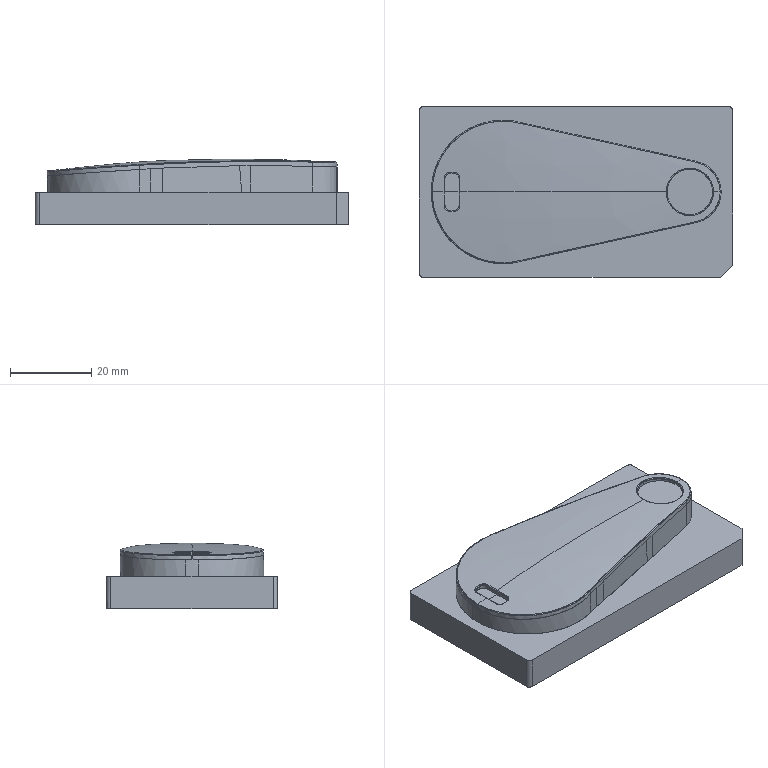NC program | PowerMill | posted with a generic post | part box 77 x 42 x 16.114 mm
Lines 5294 to 6286 of 134652:
N5391 M6
N5392 S18000 M03
N5393 G00 G90 X0.0 Y0.0
N5394 G43 Z9.8037 H2
N5395
N5396 G05 P10000 R4
N5397 X15.985 Y-10.5899
N5398 Z0.6702
N5399 G01 Z-0.5298 F3600.0
N5400 X15.9918 Y-10.569 F6000.0
N5401 G03 X15.8642 Y-10.3197 I-0.1884 J0.0609
N5402 G01 X14.5797 Y-9.9049
N5403 X12.3216 Y-10.2491
N5404 X11.9573 Y-10.2786
N5405 X10.9812 Y-10.2096
N5406 X10.4931 Y-10.2127
N5407 X7.0768 Y-10.0469
N5408 X4.1484 Y-9.3347
N5409 X3.9914 Y-9.273
N5410 X3.6604 Y-9.2133
N5411 X2.1962 Y-8.8365
N5412 X1.7082 Y-8.6326
N5413 X1.0155 Y-8.2969
N5414 X-0.244 Y-7.5021
N5415 X-2.5439 Y-5.8566
N5416 X-3.1723 Y-5.1878
N5417 X-3.8658 Y-3.9044
N5418 X-4.3321 Y-2.9283
N5419 X-4.5131 Y-2.4403
N5420 X-4.7814 Y-0.9761
N5421 X-4.9965 Y-0.4881
N5422 X-5.0691 Y0.0
N5423 X-4.9959 Y0.4881
N5424 X-4.8279 Y0.9761
N5425 X-4.5833 Y2.4403
N5426 X-4.4398 Y2.9283
N5427 X-4.1608 Y3.4164
N5428 X-3.9472 Y3.9044
N5429 X-3.6589 Y4.3925
N5430 X-2.9454 Y5.3686
N5431 X-2.4721 Y5.8566
N5432 X-1.8096 Y6.3447
N5433 X-1.7082 Y6.4511
N5434 X-0.7321 Y7.2006
N5435 X-0.6069 Y7.3208
N5436 X-0.244 Y7.5702
N5437 X0.0485 Y7.8088
N5438 X0.7321 Y8.2556
N5439 X1.2201 Y8.4464
N5440 X2.6843 Y8.9279
N5441 X3.8434 Y9.273
N5442 X4.1484 Y9.3944
N5443 X5.1246 Y9.6928
N5444 X9.517 Y10.2816
N5445 X10.0051 Y10.274
N5446 X13.9095 Y10.115
N5447 X14.3976 Y10.0238
N5448 X15.5346 Y9.7611
N5449 X15.8617 Y9.7088
N5450 X18.302 Y9.1742
N5451 X18.79 Y9.0002
N5452 X20.2542 Y8.3815
N5453 X21.2303 Y7.8837
N5454 X22.6945 Y6.9767
N5455 X23.1825 Y6.6438
N5456 X23.4753 Y6.3447
N5457 X23.6706 Y6.2105
N5458 X24.0366 Y5.8566
N5459 X24.1586 Y5.7858
N5460 X24.9777 Y4.8805
N5461 X25.1347 Y4.6324
N5462 X25.242 Y4.3925
N5463 X25.3717 Y3.9044
N5464 X25.353 Y3.4164
N5465 X25.2134 Y2.9283
N5466 X24.9263 Y2.4403
N5467 X24.4521 Y1.4642
N5468 X24.3007 Y0.9761
N5469 X24.2171 Y0.4881
N5470 X24.1864 Y0.0
N5471 X24.2177 Y-0.4881
N5472 X24.3007 Y-0.9761
N5473 X24.4552 Y-1.4642
N5474 X24.9263 Y-2.4403
N5475 X24.9304 Y-2.4473
N5476 X24.9305 Y-2.4474
N5477 X25.2136 Y-2.9283
N5478 X25.353 Y-3.4164
N5479 X25.3717 Y-3.9044
N5480 X25.242 Y-4.3925
N5481 X24.9792 Y-4.8805
N5482 X24.0229 Y-5.8566
N5483 X23.1825 Y-6.5896
N5484 X22.8614 Y-6.8327
N5485 X22.6945 Y-6.9955
N5486 X22.2064 Y-7.3451
N5487 X21.2303 Y-7.8982
N5488 X20.4067 Y-8.2969
N5489 X17.3259 Y-9.4493
N5490 X16.8378 Y-9.5607
N5491 X14.5797 Y-9.9049
N5492 X16.8369 Y-13.1705 Z-0.7226
N5493 X16.8424 Y-13.1492
N5494 G03 X16.7 Y-12.9081 I-0.1918 J0.0494
N5495 G01 X15.1386 Y-12.5061
N5496 X12.0144 Y-13.1774
N5497 X10.0051 Y-13.5276
N5498 X9.517 Y-13.568
N5499 X8.5409 Y-13.533
N5500 X7.0768 Y-13.4407
N5501 X4.6365 Y-13.0863
N5502 X2.1962 Y-12.7016
N5503 X0.7321 Y-12.2384
N5504 X-2.1962 Y-11.2009
N5505 X-2.6843 Y-10.9564
N5506 X-3.9445 Y-10.2491
N5507 X-4.6365 Y-9.7451
N5508 X-6.4624 Y-8.2969
N5509 X-7.0768 Y-7.7594
N5510 X-7.5648 Y-7.1197
N5511 X-8.6785 Y-5.3686
N5512 X-8.9342 Y-4.8805
N5513 X-9.2841 Y-3.9044
N5514 X-9.7154 Y-2.4403
N5515 X-9.9892 Y0.0
N5516 X-9.9391 Y0.4881
N5517 X-9.8428 Y0.9761
N5518 X-9.4645 Y3.4164
N5519 X-9.3065 Y3.9044
N5520 X-8.5409 Y5.4879
N5521 X-8.0529 Y6.3656
N5522 X-7.7369 Y6.8409
N5523 X-7.4278 Y7.3208
N5524 X-7.0568 Y7.8088
N5525 X-5.6126 Y9.013
N5526 X-4.0115 Y10.2491
N5527 X-3.6604 Y10.4585
N5528 X-2.6843 Y10.9644
N5529 X-0.8483 Y11.7133
N5530 X-0.7321 Y11.7403
N5531 X0.7321 Y12.3023
N5532 X1.7082 Y12.5616
N5533 X4.9711 Y13.1774
N5534 X6.1007 Y13.3217
N5535 X7.0768 Y13.4029
N5536 X8.0529 Y13.5085
N5537 X9.517 Y13.5892
N5538 X10.0051 Y13.5348
N5539 X11.9573 Y13.1885
N5540 X19.2781 Y11.6167
N5541 X24.1586 Y10.4886
N5542 X26.1108 Y9.9407
N5543 X26.4488 Y9.7611
N5544 X27.1222 Y9.273
N5545 X27.575 Y8.8486
N5546 X28.063 Y8.443
N5547 X28.683 Y7.8088
N5548 X29.4948 Y6.8327
N5549 X29.7043 Y6.3447
N5550 X29.814 Y5.8566
N5551 X29.7755 Y5.3686
N5552 X29.5272 Y4.8397
N5553 X29.1792 Y4.3925
N5554 X29.0391 Y4.301
N5555 X28.5511 Y4.0585
N5556 X27.0869 Y3.7026
N5557 X26.5989 Y3.5189
N5558 X26.1108 Y3.2616
N5559 X25.6228 Y2.9149
N5560 X25.1468 Y2.4403
N5561 X24.7984 Y1.9522
N5562 X24.5421 Y1.4642
N5563 X24.3764 Y0.9761
N5564 X24.2788 Y0.4881
N5565 X24.2425 Y0.0
N5566 X24.2788 Y-0.4881
N5567 X24.3765 Y-0.9761
N5568 X24.5432 Y-1.4642
N5569 X24.7985 Y-1.9522
N5570 X25.1347 Y-2.4286
N5571 X25.6228 Y-2.9134
N5572 X26.1108 Y-3.2612
N5573 X26.5989 Y-3.5183
N5574 X27.0869 Y-3.7067
N5575 X28.5511 Y-4.0483
N5576 X29.1791 Y-4.3925
N5577 X29.5803 Y-4.8805
N5578 X29.7754 Y-5.3686
N5579 X29.814 Y-5.8566
N5580 X29.7043 Y-6.3447
N5581 X29.5272 Y-6.7695
N5582 X29.0391 Y-7.3983
N5583 X28.6841 Y-7.8088
N5584 X28.1703 Y-8.2969
N5585 X28.063 Y-8.4416
N5586 X27.6707 Y-8.7849
N5587 X27.6697 Y-8.7859
N5588 X27.6687 Y-8.7868
N5589 X27.0869 Y-9.3106
N5590 X26.5989 Y-9.663
N5591 X26.1108 Y-9.9234
N5592 X25.6228 Y-10.0928
N5593 X24.1586 Y-10.4881
N5594 X19.2781 Y-11.6167
N5595 X15.1386 Y-12.5061
N5596 G00 Z3.4146
N5597 G01 X17.275 Y13.0315 F10000.0
N5598 G00 Z0.2846
N5599 G01 Z-0.9154 F3600.0
N5600 X17.2276 Y12.8167 F6000.0
N5601 X17.0818 Y12.1556
N5602 X24.6467 Y10.4877
N5603 X29.9536 Y9.273
N5604 X30.9913 Y8.9558
N5605 X31.9675 Y8.5409
N5606 X32.4555 Y8.2603
N5607 X32.9436 Y7.918
N5608 X33.4316 Y7.5167
N5609 X33.5949 Y7.3208
N5610 X33.8585 Y6.8327
N5611 X34.4758 Y5.3686
N5612 X34.9257 Y3.9044
N5613 X35.1649 Y2.9283
N5614 X35.2875 Y1.9522
N5615 X35.1493 Y1.4642
N5616 X34.9156 Y0.9761
N5617 X34.8958 Y0.8721
N5618 X34.4708 Y0.4881
N5619 X33.9197 Y0.215
N5620 X33.4316 Y0.1634
N5621 X32.9436 Y0.2235
N5622 X32.4555 Y0.3991
N5623 X32.4506 Y0.4188
N5624 X32.4467 Y0.4294
N5625 X32.4201 Y0.486
N5626 X32.3764 Y0.5308
N5627 X31.9675 Y0.8373
N5628 X31.4794 Y1.7222
N5629 X30.9913 Y2.3765
N5630 X30.5033 Y2.8523
N5631 X30.0152 Y3.1826
N5632 X29.5424 Y3.4164
N5633 X29.0391 Y3.6018
N5634 X28.5511 Y3.6981
N5635 X28.063 Y3.7356
N5636 X27.575 Y3.7096
N5637 X27.0869 Y3.6248
N5638 X26.5989 Y3.4707
N5639 X26.1108 Y3.2307
N5640 X25.6228 Y2.8981
N5641 X25.1347 Y2.4185
N5642 X24.7984 Y1.9522
N5643 X24.5424 Y1.4642
N5644 X24.3764 Y0.9761
N5645 X24.2788 Y0.4881
N5646 X24.2426 Y0.0
N5647 X24.2788 Y-0.4881
N5648 X24.3772 Y-0.9761
N5649 X24.5432 Y-1.4642
N5650 X24.7985 Y-1.9522
N5651 X25.1347 Y-2.4184
N5652 X25.6228 Y-2.8979
N5653 X26.1108 Y-3.2305
N5654 X26.475 Y-3.4164
N5655 X27.0869 Y-3.6228
N5656 X27.575 Y-3.7119
N5657 X28.063 Y-3.7355
N5658 X28.5511 Y-3.698
N5659 X29.0391 Y-3.6021
N5660 X29.5272 Y-3.4234
N5661 X29.7739 Y-3.3015
N5662 X28.8728 Y-1.5202
N5663 G02 X26.4134 Y-0.079 I-0.7654 J1.513
N5664 G02 X29.4882 Y0.9768 I1.694 J0.0718
N5665 G01 X29.8264 Y0.5023
N5666 G02 X29.8634 Y-0.3695 I-0.6515 J-0.4643
N5667 G01 X29.5665 Y-0.8709
N5668 G02 X28.8728 Y-1.5202 I-1.4591 J0.8636
N5669 G01 X29.7739 Y-3.3015
N5670 X30.0152 Y-3.1823
N5671 X30.4068 Y-2.9283
N5672 X30.9913 Y-2.3765
N5673 X31.4794 Y-1.7204
N5674 X31.9675 Y-0.8398
N5675 X32.3709 Y-0.5353
N5676 X32.4316 Y-0.4594
N5677 X32.4555 Y-0.3651
N5678 X32.9436 Y-0.2045
N5679 X33.4316 Y-0.1634
N5680 X33.9197 Y-0.191
N5681 X34.4077 Y-0.4074
N5682 X34.4708 Y-0.4881
N5683 X34.8958 Y-0.849
N5684 X34.9156 Y-0.9761
N5685 X35.1493 Y-1.4642
N5686 X35.2875 Y-1.9522
N5687 X35.1649 Y-2.9283
N5688 X35.0597 Y-3.4164
N5689 X34.7979 Y-4.3925
N5690 X34.4598 Y-5.3686
N5691 X34.0347 Y-6.3447
N5692 X33.8585 Y-6.8327
N5693 X33.5928 Y-7.3208
N5694 X33.4316 Y-7.5089
N5695 X33.0925 Y-7.8088
N5696 X32.4555 Y-8.2608
N5697 X31.9675 Y-8.5383
N5698 X30.9913 Y-8.9558
N5699 X30.0152 Y-9.2567
N5700 X25.1347 Y-10.3776
N5701 X16.8378 Y-12.2122
N5702 X5.6833 Y-14.6416
N5703 X3.1992 Y-15.1296
N5704 X1.7082 Y-15.3289
N5705 X0.7321 Y-15.1863
N5706 X-1.7082 Y-14.5815
N5707 X-2.6843 Y-14.2589
N5708 X-3.1723 Y-14.0252
N5709 X-6.1007 Y-12.7616
N5710 X-6.2158 Y-12.6894
N5711 X-6.5887 Y-12.5321
N5712 X-7.0768 Y-12.2223
N5713 X-7.667 Y-11.7133
N5714 X-8.827 Y-10.7372
N5715 X-9.8957 Y-9.7611
N5716 X-10.9812 Y-8.4414
N5717 X-11.0562 Y-8.2969
N5718 X-11.7166 Y-7.3208
N5719 X-11.9306 Y-6.8327
N5720 X-12.7269 Y-4.8805
N5721 X-13.2966 Y-2.4403
N5722 X-13.5318 Y0.0
N5723 X-13.1339 Y3.4164
N5724 X-13.0265 Y3.9044
N5725 X-12.8615 Y4.3925
N5726 X-12.2761 Y5.8566
N5727 X-12.055 Y6.3447
N5728 X-11.7014 Y7.3208
N5729 X-10.9812 Y8.4367
N5730 X-9.8961 Y9.7611
N5731 X-8.5409 Y11.038
N5732 X-7.5648 Y11.828
N5733 X-6.5887 Y12.5307
N5734 X-5.8996 Y12.8597
N5735 X-5.2052 Y13.1774
N5736 X-4.6365 Y13.4642
N5737 X-3.1723 Y14.0914
N5738 X-2.6843 Y14.2619
N5739 X-1.2201 Y14.7024
N5740 X0.7321 Y15.1868
N5741 X1.7082 Y15.3272
N5742 X3.1993 Y15.1296
N5743 X5.6126 Y14.6558
N5744 X9.517 Y13.8236
N5745 X17.0818 Y12.1556
N5746 X17.2276 Y12.8167
N5747 X15.8751 Y13.4159 Z-1.1082
N5748 X15.8612 Y13.3988
N5749 G03 X15.8905 Y13.1203 I0.1539 J-0.1246
N5750 G01 X17.0818 Y12.1556
N5751 X24.6467 Y10.4876
N5752 X24.6863 Y10.4785
N5753 X30.0152 Y9.3046
N5754 X30.9913 Y9.0315
N5755 X31.6504 Y8.7849
N5756 X32.6485 Y8.2969
N5757 X33.4316 Y7.7973
N5758 X33.9197 Y7.4266
N5759 X34.4077 Y7.0097
N5760 X34.8958 Y6.5253
N5761 X35.3838 Y5.9587
N5762 X35.8719 Y5.2894
N5763 X36.3599 Y4.4639
N5764 X36.6313 Y3.9044
N5765 X36.8292 Y3.4164
N5766 X37.14 Y2.4403
N5767 X37.336 Y1.4964
N5768 X37.4396 Y0.4881
N5769 Y-0.4881
N5770 X37.3407 Y-1.4642
N5771 X37.14 Y-2.4403
N5772 X36.848 Y-3.3763
N5773 X36.6333 Y-3.9044
N5774 X36.3599 Y-4.4656
N5775 X35.8719 Y-5.2895
N5776 X35.4636 Y-5.8566
N5777 X35.0579 Y-6.3447
N5778 X34.5953 Y-6.8327
N5779 X33.9197 Y-7.4274
N5780 X33.4142 Y-7.8088
N5781 X32.6481 Y-8.2969
N5782 X31.6504 Y-8.7849
N5783 X30.9913 Y-9.0294
N5784 X30.1471 Y-9.273
N5785 X22.667 Y-10.9232
N5786 X16.8378 Y-12.2122
N5787 X15.7729 Y-12.4441
N5788 X2.1962 Y-15.4393
N5789 X-1.0126 Y-16.1057
N5790 X-2.6843 Y-16.4045
N5791 X-3.6604 Y-16.4871
N5792 X-4.1484 Y-16.4057
N5793 X-6.1007 Y-15.7378
N5794 X-6.5887 Y-15.5486
N5795 X-8.0529 Y-14.7887
N5796 X-9.029 Y-14.2443
N5797 X-9.1208 Y-14.1535
N5798 X-10.4931 Y-13.2448
N5799 X-10.9812 Y-12.8331
N5800 X-11.9573 Y-11.8789
N5801 X-13.4214 Y-10.0394
N5802 X-13.9095 Y-9.3592
N5803 X-14.5184 Y-8.2969
N5804 X-14.8856 Y-7.4935
N5805 X-15.1491 Y-6.8327
N5806 X-15.2816 Y-6.3447
N5807 X-15.3737 Y-6.1218
N5808 X-15.5986 Y-5.3686
N5809 X-15.8576 Y-4.3925
N5810 X-16.21 Y-2.4403
N5811 X-16.3345 Y-0.4881
N5812 X-16.3888 Y0.0
N5813 X-16.1063 Y3.4164
N5814 X-16.004 Y3.9044
N5815 X-15.3737 Y6.0853
N5816 X-15.2688 Y6.3447
N5817 X-15.162 Y6.8327
N5818 X-14.9821 Y7.3208
N5819 X-14.5212 Y8.2969
N5820 X-14.3976 Y8.4951
N5821 X-14.267 Y8.7849
N5822 X-13.656 Y9.7611
N5823 X-12.9317 Y10.7372
N5824 X-12.4453 Y11.3284
N5825 X-11.4692 Y12.4066
N5826 X-10.5858 Y13.1774
N5827 X-9.517 Y13.9309
N5828 X-9.1208 Y14.1535
N5829 X-9.029 Y14.2299
N5830 X-8.5409 Y14.5124
N5831 X-6.5887 Y15.5482
N5832 X-6.1007 Y15.7373
N5833 X-4.1484 Y16.4125
N5834 X-3.6604 Y16.488
N5835 X-2.6843 Y16.4081
N5836 X-1.0125 Y16.1057
N5837 X1.2201 Y15.6479
N5838 X9.0502 Y13.923
N5839 X9.0508 Y13.9229
N5840 X9.517 Y13.8235
N5841 X17.0818 Y12.1556
N5842 X15.8812 Y13.4173 Z-1.301
N5843 X15.8674 Y13.4002
N5844 G03 X15.8967 Y13.1218 I0.1539 J-0.1245
N5845 G01 X17.0831 Y12.1613
N5846 X30.0152 Y9.3118
N5847 X30.5033 Y9.1853
N5848 X30.8379 Y9.0744
N5849 X30.8423 Y9.0732
N5850 X31.2509 Y8.9418
N5851 X31.6504 Y8.7849
N5852 X31.7504 Y8.736
N5853 X32.4555 Y8.4084
N5854 X32.9436 Y8.1319
N5855 X33.4337 Y7.8088
N5856 X34.0717 Y7.3208
N5857 X34.3732 Y7.0391
N5858 X34.4077 Y7.0097
N5859 X34.4548 Y6.963
N5860 X34.8958 Y6.551
N5861 X35.3838 Y5.9928
N5862 X35.8719 Y5.3332
N5863 X36.3599 Y4.5207
N5864 X36.6659 Y3.9044
N5865 X36.848 Y3.4634
N5866 X37.1824 Y2.4403
N5867 X37.3851 Y1.4642
N5868 X37.487 Y0.4881
N5869 X37.4872 Y-0.4881
N5870 X37.3871 Y-1.4642
N5871 X37.1852 Y-2.4403
N5872 X37.0358 Y-2.9283
N5873 X36.6659 Y-3.9044
N5874 X36.3599 Y-4.5218
N5875 X35.8457 Y-5.3686
N5876 X35.4887 Y-5.8566
N5877 X34.8958 Y-6.551
N5878 X34.6122 Y-6.8327
N5879 X34.0705 Y-7.3208
N5880 X33.4316 Y-7.8121
N5881 X32.9436 Y-8.1319
N5882 X32.4555 Y-8.4084
N5883 X31.6685 Y-8.7849
N5884 X30.9913 Y-9.0374
N5885 X30.0152 Y-9.3119
N5886 X-3.0263 Y-16.5938
N5887 X-5.3877 Y-17.0818
N5888 X-7.0768 Y-17.3569
N5889 X-7.5648 Y-17.3933
N5890 X-8.0529 Y-17.3741
N5891 X-8.5409 Y-17.2194
N5892 X-9.8825 Y-16.5938
N5893 X-10.4931 Y-16.2662
N5894 X-11.5234 Y-15.6177
N5895 X-12.8694 Y-14.6416
N5896 X-13.4893 Y-14.1535
N5897 X-14.388 Y-13.1774
N5898 X-15.5219 Y-11.7133
N5899 X-16.3498 Y-10.2735
N5900 X-16.6683 Y-9.7611
N5901 X-16.9285 Y-9.273
N5902 X-17.8139 Y-7.1013
N5903 X-17.8962 Y-6.8327
N5904 X-17.9805 Y-6.3447
N5905 X-18.2202 Y-5.3686
N5906 X-18.4325 Y-4.3925
N5907 X-18.7084 Y-2.4403
N5908 X-18.8098 Y-0.4881
N5909 X-18.8636 Y0.0
N5910 X-18.6188 Y3.4164
N5911 X-18.5192 Y3.9044
N5912 X-17.9635 Y6.3447
N5913 X-17.8966 Y6.8327
N5914 X-17.8139 Y7.1013
N5915 X-17.3259 Y8.3813
N5916 X-16.9288 Y9.273
N5917 X-16.1465 Y10.7372
N5918 X-15.5346 Y11.7133
N5919 X-15.196 Y12.2013
N5920 X-14.8856 Y12.5959
N5921 X-13.9095 Y13.7109
N5922 X-12.4453 Y14.9669
N5923 X-11.5309 Y15.6177
N5924 X-10.4931 Y16.289
N5925 X-8.5409 Y17.224
N5926 X-8.0529 Y17.3748
N5927 X-7.5648 Y17.3896
N5928 X-7.0768 Y17.3569
N5929 X-5.6126 Y17.1212
N5930 X-3.1723 Y16.6245
N5931 X17.0831 Y12.1613
N5932 X15.87 Y13.4318 Z-1.4939
N5933 X15.8561 Y13.4147
N5934 G03 X15.8855 Y13.1363 I0.154 J-0.1245
N5935 G01 X17.0842 Y12.1662
N5936 X30.0152 Y9.3187
N5937 X30.5033 Y9.1912
N5938 X30.9652 Y9.0388
N5939 X30.9913 Y9.0314
N5940 X31.0211 Y9.0203
N5941 X31.4794 Y8.8691
N5942 X32.4555 Y8.4161
N5943 X32.9436 Y8.1397
N5944 X33.4417 Y7.8088
N5945 X33.9197 Y7.4538
N5946 X34.4077 Y7.0364
N5947 X34.8958 Y6.5609
N5948 X35.3838 Y6.0032
N5949 X35.8554 Y5.3686
N5950 X36.3599 Y4.5357
N5951 X36.6741 Y3.9044
N5952 X36.8711 Y3.4164
N5953 X37.1923 Y2.4403
N5954 X37.336 Y1.79
N5955 X37.3789 Y1.4936
N5956 X37.385 Y1.4642
N5957 X37.3898 Y1.4181
N5958 X37.4538 Y0.9761
N5959 X37.4754 Y0.5983
N5960 X37.4866 Y0.4952
N5961 X37.4873 Y0.3916
N5962 X37.5097 Y0.0
N5963 X37.4927 Y-0.4881
N5964 X37.3944 Y-1.4642
N5965 X37.1922 Y-2.4403
N5966 X37.045 Y-2.9283
N5967 X36.6741 Y-3.9044
N5968 X36.3599 Y-4.536
N5969 X35.8719 Y-5.3449
N5970 X35.4966 Y-5.8566
N5971 X34.8958 Y-6.5608
N5972 X34.4077 Y-7.0366
N5973 X34.0809 Y-7.3208
N5974 X33.4464 Y-7.8088
N5975 X32.9436 Y-8.1397
N5976 X32.4555 Y-8.4161
N5977 X31.6849 Y-8.7849
N5978 X30.9913 Y-9.0449
N5979 X30.0152 Y-9.3187
N5980 X-7.4559 Y-17.5699
N5981 X-9.029 Y-17.8917
N5982 X-9.76 Y-18.0169
N5983 X-10.4931 Y-18.1296
N5984 X-10.9812 Y-18.1485
N5985 X-11.4692 Y-18.1366
N5986 X-11.7996 Y-18.0579
N5987 X-11.9573 Y-17.9896
N5988 X-12.9334 Y-17.4587
N5989 X-14.8113 Y-16.1057
N5990 X-15.4001 Y-15.6177
N5991 X-16.3591 Y-14.6416
N5992 X-17.1793 Y-13.6655
N5993 X-17.5114 Y-13.1774
N5994 X-18.3798 Y-11.7133
N5995 X-18.6318 Y-11.2252
N5996 X-18.8262 Y-10.7372
N5997 X-19.4761 Y-9.273
N5998 X-20.2686 Y-6.8327
N5999 X-20.7217 Y-4.3925
N6000 X-20.9442 Y-2.4403
N6001 X-21.0669 Y0.0
N6002 X-20.8559 Y3.4164
N6003 X-20.2594 Y6.8327
N6004 X-19.9799 Y7.8088
N6005 X-19.6459 Y8.7849
N6006 X-19.0892 Y10.2491
N6007 X-18.393 Y11.7133
N6008 X-17.8139 Y12.7014
N6009 X-17.3259 Y13.448
N6010 X-16.3341 Y14.6416
N6011 X-15.878 Y15.1296
N6012 X-14.8856 Y16.0714
N6013 X-13.9095 Y16.8229
N6014 X-12.4453 Y17.7241
N6015 X-11.9573 Y17.9898
N6016 X-11.4692 Y18.1338
N6017 X-10.9812 Y18.1508
N6018 X-10.4931 Y18.1286
N6019 X-9.029 Y17.8905
N6020 X-7.4559 Y17.5699
N6021 X17.0842 Y12.1662
N6022 X15.8638 Y13.4435 Z-1.6867
N6023 X15.85 Y13.4264
N6024 G03 X15.8794 Y13.1479 I0.1539 J-0.1246
N6025 G01 X17.0854 Y12.1719
N6026 X30.0152 Y9.3256
N6027 X30.5033 Y9.1981
N6028 X31.4794 Y8.8762
N6029 X32.4555 Y8.4238
N6030 X32.9436 Y8.1475
N6031 X33.1484 Y8.0036
N6032 X33.1505 Y8.0022
N6033 X33.5386 Y7.7369
N6034 X33.9197 Y7.4616
N6035 X34.4077 Y7.0459
N6036 X34.8958 Y6.5707
N6037 X35.3838 Y6.0136
N6038 X35.8636 Y5.3686
N6039 X36.3599 Y4.5507
N6040 X36.6817 Y3.9044
N6041 X36.8786 Y3.4164
N6042 X37.1993 Y2.4403
N6043 X37.336 Y1.822
N6044 X37.4594 Y0.9761
N6045 X37.5165 Y0.0
N6046 X37.4967 Y-0.3735
N6047 X37.4927 Y-0.488
N6048 X37.4883 Y-0.5317
N6049 X37.4647 Y-0.9761
N6050 X37.4014 Y-1.4642
N6051 X37.1992 Y-2.4403
N6052 X37.0519 Y-2.9283
N6053 X36.6817 Y-3.9044
N6054 X36.3599 Y-4.5512
N6055 X35.8719 Y-5.3566
N6056 X35.505 Y-5.8566
N6057 X34.8958 Y-6.5707
N6058 X34.4963 Y-6.9486
N6059 X34.0913 Y-7.3208
N6060 X33.4316 Y-7.8245
N6061 X32.9436 Y-8.1475
N6062 X32.4555 Y-8.4238
N6063 X31.7014 Y-8.7849
N6064 X30.9913 Y-9.052
N6065 X30.0152 Y-9.3256
N6066 X-10.0051 Y-18.1367
N6067 X-11.9652 Y-18.546
N6068 X-13.4214 Y-18.8225
N6069 X-13.9095 Y-18.8456
N6070 X-14.3976 Y-18.8271
N6071 X-14.8856 Y-18.6811
N6072 X-15.1294 Y-18.546
N6073 X-15.8617 Y-18.0621
N6074 X-16.8378 Y-17.3034
N6075 X-18.5155 Y-15.6177
N6076 X-18.9206 Y-15.1296
N6077 X-19.8962 Y-13.6655
N6078 X-20.7422 Y-12.0263
N6079 X-21.0951 Y-11.2252
N6080 X-21.2683 Y-10.7372
N6081 X-21.9133 Y-8.7849
N6082 X-22.2064 Y-7.5947
N6083 X-22.4226 Y-6.8327
N6084 X-22.818 Y-4.3925
N6085 X-23.0036 Y-2.4403
N6086 X-23.1023 Y0.0
N6087 X-22.9211 Y3.4164
N6088 X-22.6748 Y5.1258
N6089 X-22.4117 Y6.8327
N6090 X-22.3032 Y7.3208
N6091 X-21.7183 Y9.4498
N6092 X-21.0951 Y11.2252
N6093 X-20.8839 Y11.7133
N6094 X-20.1615 Y13.1774
N6095 X-19.2498 Y14.6416
N6096 X-18.302 Y15.867
N6097 X-18.0833 Y16.1057
N6098 X-17.1188 Y17.0818
N6099 X-15.1394 Y18.546
N6100 X-14.8856 Y18.673
N6101 X-14.3976 Y18.826
N6102 X-13.9095 Y18.8467
N6103 X-13.4214 Y18.8227
N6104 X-10.4931 Y18.2429
N6105 X17.0854 Y12.1719
N6106 X15.8776 Y13.4394 Z-1.8852
N6107 X15.8637 Y13.4223
N6108 G03 X15.8931 Y13.1438 I0.1539 J-0.1245
N6109 G01 X17.0868 Y12.178
N6110 X30.0152 Y9.3327
N6111 X30.5033 Y9.2053
N6112 X31.4794 Y8.8835
N6113 X32.4555 Y8.4318
N6114 X32.9436 Y8.1556
N6115 X33.4316 Y7.8312
N6116 X33.9197 Y7.4694
N6117 X34.4077 Y7.0557
N6118 X34.8958 Y6.5808
N6119 X35.3838 Y6.0244
N6120 X35.8719 Y5.369
N6121 X36.3599 Y4.5661
N6122 X36.6892 Y3.9044
N6123 X36.8862 Y3.4164
N6124 X37.2065 Y2.4403
N6125 X37.3129 Y1.9262
N6126 X37.336 Y1.8219
N6127 X37.3395 Y1.7979
N6128 X37.3407 Y1.7922
N6129 X37.4086 Y1.4642
N6130 X37.4664 Y0.9761
N6131 X37.5234 Y0.0
N6132 X37.5055 Y-0.4881
N6133 X37.4604 Y-0.9764
N6134 X37.4086 Y-1.4642
N6135 X37.2064 Y-2.4403
N6136 X37.059 Y-2.9283
N6137 X36.6892 Y-3.9044
N6138 X36.3599 Y-4.5668
N6139 X35.8719 Y-5.3687
N6140 X35.5136 Y-5.8566
N6141 X34.8958 Y-6.5808
N6142 X34.443 Y-7.0021
N6143 X34.4076 Y-7.0366
N6144 X34.3818 Y-7.059
N6145 X34.1005 Y-7.3208
N6146 X33.4644 Y-7.8088
N6147 X32.9436 Y-8.1556
N6148 X32.4555 Y-8.4318
N6149 X31.7183 Y-8.7849
N6150 X30.9913 Y-9.0594
N6151 X30.0152 Y-9.3327
N6152 X-12.4453 Y-18.6768
N6153 X-13.8798 Y-19.0341
N6154 X-14.8856 Y-19.2036
N6155 X-15.8617 Y-19.2952
N6156 X-16.8378 Y-19.3065
N6157 X-17.3259 Y-19.2432
N6158 X-17.8139 Y-19.1043
N6159 X-17.9671 Y-19.0341
N6160 X-18.302 Y-18.7971
N6161 X-18.79 Y-18.397
N6162 X-19.6715 Y-17.5699
N6163 X-20.2542 Y-16.9312
N6164 X-21.5924 Y-15.1296
N6165 X-22.5928 Y-13.1774
N6166 X-23.3677 Y-11.2252
N6167 X-23.5299 Y-10.7372
N6168 X-24.0651 Y-8.7849
N6169 X-24.5739 Y-6.3447
N6170 X-24.8489 Y-4.3925
N6171 X-25.0099 Y-2.4403
N6172 X-25.0839 Y0.0
N6173 X-24.9361 Y3.4164
N6174 X-24.5668 Y6.3447
N6175 X-24.3906 Y7.3208
N6176 X-24.0672 Y8.7849
N6177 X-23.531 Y10.7372
N6178 X-23.3678 Y11.2252
N6179 X-22.7967 Y12.6894
N6180 X-22.1082 Y14.1535
N6181 X-21.5589 Y15.1296
N6182 X-21.2303 Y15.6613
N6183 X-20.2542 Y16.9747
N6184 X-18.302 Y18.8092
N6185 X-17.9729 Y19.0341
N6186 X-17.8139 Y19.1056
N6187 X-17.3259 Y19.2381
N6188 X-16.8378 Y19.3072
N6189 X-16.3498 Y19.3149
N6190 X-15.3737 Y19.2642
N6191 X-13.8851 Y19.0341
N6192 X-12.4453 Y18.6774
N6193 X17.0868 Y12.178
N6194 X15.8856 Y13.44 Z-2.0838
N6195 X15.8718 Y13.4229
N6196 G03 X15.9011 Y13.1444 I0.1539 J-0.1246
N6197 G01 X17.0881 Y12.184
N6198 X30.0152 Y9.3386
N6199 X30.5033 Y9.2144
N6200 X31.4794 Y8.8911
N6201 X32.4555 Y8.4398
N6202 X32.9436 Y8.1637
N6203 X33.4316 Y7.8396
N6204 X33.8241 Y7.5402
N6205 X33.9196 Y7.4693
N6206 X33.9439 Y7.4487
N6207 X34.3093 Y7.1437
N6208 X34.6542 Y6.8158
N6209 X34.8958 Y6.591
N6210 X35.3838 Y6.0351
N6211 X35.8719 Y5.3809
N6212 X36.3599 Y4.5816
N6213 X36.6968 Y3.9044
N6214 X36.8939 Y3.4164
N6215 X37.2137 Y2.4403
N6216 X37.326 Y1.9522
N6217 X37.3809 Y1.5976
N6218 X37.4131 Y1.4358
N6219 X37.4313 Y1.2719
N6220 X37.4771 Y0.9761
N6221 X37.5303 Y0.0
N6222 X37.5131 Y-0.4881
N6223 X37.4648 Y-0.9733
N6224 X37.4646 Y-0.9761
N6225 X37.4641 Y-0.9804
N6226 X37.4159 Y-1.4642
N6227 X37.2136 Y-2.4403
N6228 X37.0661 Y-2.9283
N6229 X36.6968 Y-3.9044
N6230 X36.3599 Y-4.5824
N6231 X35.8806 Y-5.3686
N6232 X35.5222 Y-5.8566
N6233 X34.8958 Y-6.591
N6234 X34.1116 Y-7.3208
N6235 X33.4767 Y-7.8088
N6236 X32.9436 Y-8.1637
N6237 X32.4555 Y-8.4397
N6238 X31.7352 Y-8.7849
N6239 X30.9913 Y-9.0664
N6240 X30.0152 Y-9.3386
N6241 X3.1723 Y-15.2626
N6242 X-12.4453 Y-18.6845
N6243 X-13.8388 Y-19.0341
N6244 X-15.3737 Y-19.2963
N6245 X-16.8378 Y-19.4324
N6246 X-17.8139 Y-19.4542
N6247 X-18.79 Y-19.4163
N6248 X-19.2781 Y-19.359
N6249 X-20.2542 Y-19.1993
N6250 X-20.7832 Y-19.0341
N6251 X-21.2303 Y-18.8056
N6252 X-21.7183 Y-18.3472
N6253 X-22.3694 Y-17.5699
N6254 X-23.0863 Y-16.5938
N6255 X-23.9567 Y-15.1296
N6256 X-24.1586 Y-14.7195
N6257 X-24.8063 Y-13.1774
N6258 X-25.6023 Y-10.7372
N6259 X-26.1007 Y-8.7849
N6260 X-26.4667 Y-6.8327
N6261 X-26.7929 Y-4.3925
N6262 X-26.9389 Y-2.4403
N6263 X-27.0116 Y0.0
N6264 X-26.8768 Y3.4164
N6265 X-26.5411 Y6.3447
N6266 X-26.1009 Y8.7849
N6267 X-25.6228 Y10.6524
N6268 X-25.1347 Y12.2447
N6269 X-24.6467 Y13.5339
N6270 X-23.945 Y15.1296
N6271 X-23.1825 Y16.4798
N6272 X-22.7403 Y17.0818
N6273 X-21.9738 Y18.0579
N6274 X-21.5367 Y18.546
N6275 X-21.2303 Y18.8076
N6276 X-20.783 Y19.0341
N6277 X-20.2542 Y19.2038
N6278 X-19.7661 Y19.2973
N6279 X-18.79 Y19.4125
N6280 X-17.8139 Y19.4518
N6281 X-16.8378 Y19.4329
N6282 X-15.3737 Y19.2964
N6283 X-13.9095 Y19.0492
N6284 X-12.4453 Y18.6845
N6285 X-12.4427 Y18.6839
N6286 X17.0881 Y12.184
N6287 X15.8932 Y13.4366 Z-2.2824
N6288 X15.8793 Y13.4195
N6289 G03 X15.9087 Y13.141 I0.1539 J-0.1246
N6290 G01 X17.0885 Y12.186
N6291 X30.0152 Y9.3386
N6292 X30.0175 Y9.338
N6293 X30.5033 Y9.2144
N6294 X30.7304 Y9.1392
N6295 X30.7349 Y9.1379
N6296 X30.9913 Y9.0664
N6297 X31.3656 Y8.9288
N6298 X31.7374 Y8.7849
N6299 X32.0941 Y8.6074
N6300 X32.4555 Y8.4397
N6301 X32.5862 Y8.3647
N6302 X32.7207 Y8.2969
N6303 X33.0794 Y8.0746
N6304 X33.4316 Y7.842
N6305 X34.1169 Y7.3208
N6306 X34.342 Y7.1113
N6307 X34.4076 Y7.0556
N6308 X34.5377 Y6.9291
N6309 X34.8958 Y6.5958
N6310 X35.3838 Y6.0407
N6311 X35.8719 Y5.3883
N6312 X36.3599 Y4.5929
N6313 X36.7023 Y3.9044
N6314 X36.9002 Y3.4164
N6315 X37.2194 Y2.4403
N6316 X37.272 Y2.1868
N6317 X37.326 Y1.9522
N6318 X37.3417 Y1.8507
N6319 X37.4219 Y1.4642
N6320 X37.463 Y1.0668
N6321 X37.4772 Y0.9744
N6322 X37.4822 Y0.8812
N6323 X37.5229 Y0.4881
N6324 X37.5228 Y0.1383
N6325 X37.5303 Y0.0
N6326 X37.5221 Y-0.244
N6327 X37.5225 Y-0.4881
N6328 X37.422 Y-1.4642
N6329 X37.2194 Y-2.4403
N6330 X37.0716 Y-2.9283
N6331 X36.7023 Y-3.9044
N6332 X36.3599 Y-4.593
N6333 X35.8858 Y-5.3686
N6334 X35.5289 Y-5.8566
N6335 X34.8958 Y-6.5958
N6336 X34.1167 Y-7.3208
N6337 X33.4803 Y-7.8088
N6338 X33.1041 Y-8.0586
N6339 X32.7205 Y-8.2969
N6340 X32.5861 Y-8.3647
N6341 X32.4555 Y-8.4396
N6342 X31.8321 Y-8.7384
N6343 X31.7385 Y-8.7849
N6344 X30.9913 Y-9.0664
N6345 X30.0152 Y-9.3386
N6346 X29.8857 Y-9.3671
N6347 X3.1723 Y-15.2626
N6348 X-6.3434 Y-17.3475
N6349 X-12.4453 Y-18.6916
N6350 X-13.8076 Y-19.0341
N6351 X-15.3737 Y-19.3058
N6352 X-16.8378 Y-19.442
N6353 X-17.8139 Y-19.4702
N6354 X-18.79 Y-19.4473
N6355 X-20.2542 Y-19.3296
N6356 X-21.2303 Y-19.1765
N6357 X-22.2064 Y-18.9627
N6358 X-23.4957 Y-18.546
N6359 X-24.1586 Y-18.197
N6360 X-24.3522 Y-18.0579
N6361 X-24.6467 Y-17.7465
N6362 X-25.1347 Y-17.0114
N6363 X-25.3706 Y-16.5938
N6364 X-26.3436 Y-14.6416
N6365 X-26.876 Y-13.1774
N6366 X-27.592 Y-10.7372
N6367 X-28.039 Y-8.7849
N6368 X-28.4566 Y-6.3447
N6369 X-28.6986 Y-4.3925
N6370 X-28.8334 Y-2.4403
N6371 X-28.9135 Y0.0
N6372 X-28.8668 Y1.9522
N6373 X-28.7829 Y3.4164
N6374 X-28.456 Y6.3447
N6375 X-28.1336 Y8.2969
N6376 X-27.5926 Y10.7372
N6377 X-27.0298 Y12.6894
N6378 X-26.338 Y14.6416
N6379 X-26.1229 Y15.1296
N6380 X-25.6228 Y16.1463
N6381 X-25.3713 Y16.5938
N6382 X-24.6467 Y17.7535
N6383 X-24.3539 Y18.0579